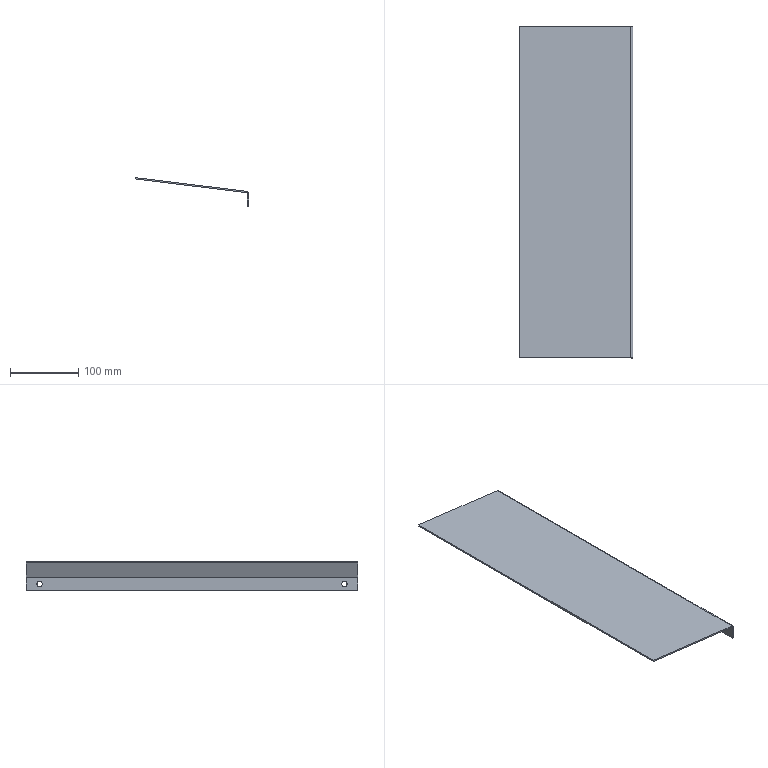Part | STEP file | JBJ-P-1006-09 | 1 solid | 16 faces | box 167 x 488 x 42.231 mm | volume 182511 mm3 | plane 12 | cylinder 4 | commonest cylinder face diameters 8 x2 3 x1 7 x1
STEP:
#1=CARTESIAN_POINT('',(163.,488.,-1.327));
#2=VERTEX_POINT('',#1);
#3=CARTESIAN_POINT('',(165.,488.,-1.327));
#4=VERTEX_POINT('',#3);
#5=CARTESIAN_POINT('',(163.,488.,-1.327));
#6=DIRECTION('',(1.,0.,0.));
#7=VECTOR('',#6,1000.);
#8=LINE('',#5,#7);
#9=EDGE_CURVE('',#2,#4,#8,.T.);
#10=ORIENTED_EDGE('',*,*,#9,.F.);
#11=CARTESIAN_POINT('',(161.683,488.,0.1616));
#12=VERTEX_POINT('',#11);
#13=CARTESIAN_POINT('',(161.5,488.,-1.327));
#14=DIRECTION('',(0.,1.,0.));
#15=DIRECTION('',(0.,0.,-1.));
#16=AXIS2_PLACEMENT_3D('',#13,#14,#15);
#17=CIRCLE('',#16,1.5);
#18=EDGE_CURVE('',#12,#2,#17,.T.);
#19=ORIENTED_EDGE('',*,*,#18,.F.);
#20=CARTESIAN_POINT('',(161.926,488.,2.147));
#21=VERTEX_POINT('',#20);
#22=CARTESIAN_POINT('',(161.926,488.,2.147));
#23=DIRECTION('',(-0.1218,0.,-0.9926));
#24=VECTOR('',#23,1000.);
#25=LINE('',#22,#24);
#26=EDGE_CURVE('',#21,#12,#25,.T.);
#27=ORIENTED_EDGE('',*,*,#26,.F.);
#28=CARTESIAN_POINT('',(161.5,488.,-1.327));
#29=DIRECTION('',(0.,1.,0.));
#30=DIRECTION('',(1.,0.,0.));
#31=AXIS2_PLACEMENT_3D('',#28,#29,#30);
#32=CIRCLE('',#31,3.5);
#33=EDGE_CURVE('',#21,#4,#32,.T.);
#34=ORIENTED_EDGE('',*,*,#33,.T.);
#35=EDGE_LOOP('',(#10,#19,#27,#34));
#36=FACE_OUTER_BOUND('',#35,.T.);
#37=CARTESIAN_POINT('',(163.,488.,-1.327));
#38=DIRECTION('',(0.,1.,0.));
#39=DIRECTION('',(0.,0.,1.));
#40=AXIS2_PLACEMENT_3D('',#37,#38,#39);
#41=PLANE('',#40);
#42=ADVANCED_FACE('',(#36),#41,.T.);
#43=CARTESIAN_POINT('',(163.,488.,-20.));
#44=VERTEX_POINT('',#43);
#45=CARTESIAN_POINT('',(163.,488.,0.));
#46=DIRECTION('',(0.,0.,-1.));
#47=VECTOR('',#46,1000.);
#48=LINE('',#45,#47);
#49=EDGE_CURVE('',#2,#44,#48,.T.);
#50=ORIENTED_EDGE('',*,*,#49,.F.);
#51=ORIENTED_EDGE('',*,*,#9,.T.);
#52=CARTESIAN_POINT('',(165.,488.,-20.));
#53=VERTEX_POINT('',#52);
#54=CARTESIAN_POINT('',(165.,488.,0.));
#55=DIRECTION('',(0.,0.,-1.));
#56=VECTOR('',#55,1000.);
#57=LINE('',#54,#56);
#58=EDGE_CURVE('',#4,#53,#57,.T.);
#59=ORIENTED_EDGE('',*,*,#58,.T.);
#60=CARTESIAN_POINT('',(163.,488.,-20.));
#61=DIRECTION('',(1.,0.,0.));
#62=VECTOR('',#61,1000.);
#63=LINE('',#60,#62);
#64=EDGE_CURVE('',#44,#53,#63,.T.);
#65=ORIENTED_EDGE('',*,*,#64,.F.);
#66=EDGE_LOOP('',(#50,#51,#59,#65));
#67=FACE_OUTER_BOUND('',#66,.T.);
#68=CARTESIAN_POINT('',(161.926,488.,2.147));
#69=DIRECTION('',(0.,1.,0.));
#70=DIRECTION('',(0.,0.,1.));
#71=AXIS2_PLACEMENT_3D('',#68,#69,#70);
#72=PLANE('',#71);
#73=ADVANCED_FACE('',(#67),#72,.T.);
#74=CARTESIAN_POINT('',(161.683,0.,0.1616));
#75=VERTEX_POINT('',#74);
#76=CARTESIAN_POINT('',(161.926,0.,2.147));
#77=VERTEX_POINT('',#76);
#78=CARTESIAN_POINT('',(161.683,0.,0.1616));
#79=DIRECTION('',(0.1218,0.,0.9926));
#80=VECTOR('',#79,1000.);
#81=LINE('',#78,#80);
#82=EDGE_CURVE('',#75,#77,#81,.T.);
#83=ORIENTED_EDGE('',*,*,#82,.F.);
#84=CARTESIAN_POINT('',(163.,0.,-1.327));
#85=VERTEX_POINT('',#84);
#86=CARTESIAN_POINT('',(161.5,0.,-1.327));
#87=DIRECTION('',(0.,1.,0.));
#88=DIRECTION('',(0.,0.,-1.));
#89=AXIS2_PLACEMENT_3D('',#86,#87,#88);
#90=CIRCLE('',#89,1.5);
#91=EDGE_CURVE('',#75,#85,#90,.T.);
#92=ORIENTED_EDGE('',*,*,#91,.T.);
#93=CARTESIAN_POINT('',(165.,0.,-1.327));
#94=VERTEX_POINT('',#93);
#95=CARTESIAN_POINT('',(165.,0.,-1.327));
#96=DIRECTION('',(-1.,0.,0.));
#97=VECTOR('',#96,1000.);
#98=LINE('',#95,#97);
#99=EDGE_CURVE('',#94,#85,#98,.T.);
#100=ORIENTED_EDGE('',*,*,#99,.F.);
#101=CARTESIAN_POINT('',(161.5,0.,-1.327));
#102=DIRECTION('',(0.,1.,0.));
#103=DIRECTION('',(1.,0.,0.));
#104=AXIS2_PLACEMENT_3D('',#101,#102,#103);
#105=CIRCLE('',#104,3.5);
#106=EDGE_CURVE('',#77,#94,#105,.T.);
#107=ORIENTED_EDGE('',*,*,#106,.F.);
#108=EDGE_LOOP('',(#83,#92,#100,#107));
#109=FACE_OUTER_BOUND('',#108,.T.);
#110=CARTESIAN_POINT('',(161.683,0.,0.1616));
#111=DIRECTION('',(0.,-1.,0.));
#112=DIRECTION('',(0.,0.,-1.));
#113=AXIS2_PLACEMENT_3D('',#110,#111,#112);
#114=PLANE('',#113);
#115=ADVANCED_FACE('',(#109),#114,.T.);
#116=CARTESIAN_POINT('',(-2.,0.,20.245));
#117=VERTEX_POINT('',#116);
#118=CARTESIAN_POINT('',(-2.,0.,20.245));
#119=DIRECTION('',(0.9926,0.,-0.1218));
#120=VECTOR('',#119,1000.);
#121=LINE('',#118,#120);
#122=EDGE_CURVE('',#117,#75,#121,.T.);
#123=ORIENTED_EDGE('',*,*,#122,.T.);
#124=ORIENTED_EDGE('',*,*,#82,.T.);
#125=CARTESIAN_POINT('',(-1.756,0.,22.231));
#126=VERTEX_POINT('',#125);
#127=CARTESIAN_POINT('',(-1.756,0.,22.231));
#128=DIRECTION('',(0.9926,0.,-0.1218));
#129=VECTOR('',#128,1000.);
#130=LINE('',#127,#129);
#131=EDGE_CURVE('',#126,#77,#130,.T.);
#132=ORIENTED_EDGE('',*,*,#131,.F.);
#133=CARTESIAN_POINT('',(-1.756,0.,22.231));
#134=DIRECTION('',(-0.1218,0.,-0.9926));
#135=VECTOR('',#134,1000.);
#136=LINE('',#133,#135);
#137=EDGE_CURVE('',#126,#117,#136,.T.);
#138=ORIENTED_EDGE('',*,*,#137,.T.);
#139=EDGE_LOOP('',(#123,#124,#132,#138));
#140=FACE_OUTER_BOUND('',#139,.T.);
#141=CARTESIAN_POINT('',(165.,0.,-1.327));
#142=DIRECTION('',(0.,-1.,0.));
#143=DIRECTION('',(0.,0.,-1.));
#144=AXIS2_PLACEMENT_3D('',#141,#142,#143);
#145=PLANE('',#144);
#146=ADVANCED_FACE('',(#140),#145,.T.);
#147=CARTESIAN_POINT('',(165.,468.,-6.664));
#148=VERTEX_POINT('',#147);
#149=CARTESIAN_POINT('',(165.,468.,-10.664));
#150=DIRECTION('',(-1.,0.,0.));
#151=DIRECTION('',(0.,0.,1.));
#152=AXIS2_PLACEMENT_3D('',#149,#150,#151);
#153=CIRCLE('',#152,4.);
#154=EDGE_CURVE('',#148,#148,#153,.T.);
#155=ORIENTED_EDGE('',*,*,#154,.T.);
#156=EDGE_LOOP('',(#155));
#157=FACE_BOUND('',#156,.T.);
#158=CARTESIAN_POINT('',(165.,20.,-6.664));
#159=VERTEX_POINT('',#158);
#160=CARTESIAN_POINT('',(165.,20.,-10.664));
#161=DIRECTION('',(-1.,0.,0.));
#162=DIRECTION('',(0.,0.,1.));
#163=AXIS2_PLACEMENT_3D('',#160,#161,#162);
#164=CIRCLE('',#163,4.);
#165=EDGE_CURVE('',#159,#159,#164,.T.);
#166=ORIENTED_EDGE('',*,*,#165,.T.);
#167=EDGE_LOOP('',(#166));
#168=FACE_BOUND('',#167,.T.);
#169=CARTESIAN_POINT('',(165.,0.,-20.));
#170=VERTEX_POINT('',#169);
#171=CARTESIAN_POINT('',(165.,0.,0.));
#172=DIRECTION('',(0.,0.,-1.));
#173=VECTOR('',#172,1000.);
#174=LINE('',#171,#173);
#175=EDGE_CURVE('',#94,#170,#174,.T.);
#176=ORIENTED_EDGE('',*,*,#175,.T.);
#177=CARTESIAN_POINT('',(165.,488.,-20.));
#178=DIRECTION('',(0.,-1.,0.));
#179=VECTOR('',#178,1000.);
#180=LINE('',#177,#179);
#181=EDGE_CURVE('',#53,#170,#180,.T.);
#182=ORIENTED_EDGE('',*,*,#181,.F.);
#183=ORIENTED_EDGE('',*,*,#58,.F.);
#184=CARTESIAN_POINT('',(165.,488.,-1.327));
#185=DIRECTION('',(0.,-1.,0.));
#186=VECTOR('',#185,1000.);
#187=LINE('',#184,#186);
#188=EDGE_CURVE('',#4,#94,#187,.T.);
#189=ORIENTED_EDGE('',*,*,#188,.T.);
#190=EDGE_LOOP('',(#176,#182,#183,#189));
#191=FACE_OUTER_BOUND('',#190,.T.);
#192=CARTESIAN_POINT('',(165.,488.,0.));
#193=DIRECTION('',(-1.,0.,0.));
#194=DIRECTION('',(0.,0.,1.));
#195=AXIS2_PLACEMENT_3D('',#192,#193,#194);
#196=PLANE('',#195);
#197=ADVANCED_FACE('',(#157,#168,#191),#196,.F.);
#198=CARTESIAN_POINT('',(163.,0.,-20.));
#199=VERTEX_POINT('',#198);
#200=CARTESIAN_POINT('',(163.,0.,-20.));
#201=DIRECTION('',(1.,0.,0.));
#202=VECTOR('',#201,1000.);
#203=LINE('',#200,#202);
#204=EDGE_CURVE('',#199,#170,#203,.T.);
#205=ORIENTED_EDGE('',*,*,#204,.F.);
#206=CARTESIAN_POINT('',(163.,488.,-20.));
#207=DIRECTION('',(0.,-1.,0.));
#208=VECTOR('',#207,1000.);
#209=LINE('',#206,#208);
#210=EDGE_CURVE('',#44,#199,#209,.T.);
#211=ORIENTED_EDGE('',*,*,#210,.F.);
#212=ORIENTED_EDGE('',*,*,#64,.T.);
#213=ORIENTED_EDGE('',*,*,#181,.T.);
#214=EDGE_LOOP('',(#205,#211,#212,#213));
#215=FACE_OUTER_BOUND('',#214,.T.);
#216=CARTESIAN_POINT('',(163.,488.,-20.));
#217=DIRECTION('',(0.,0.,-1.));
#218=DIRECTION('',(-1.,0.,0.));
#219=AXIS2_PLACEMENT_3D('',#216,#217,#218);
#220=PLANE('',#219);
#221=ADVANCED_FACE('',(#215),#220,.T.);
#222=CARTESIAN_POINT('',(163.,468.,-6.664));
#223=VERTEX_POINT('',#222);
#224=CARTESIAN_POINT('',(163.,468.,-10.664));
#225=DIRECTION('',(-1.,0.,0.));
#226=DIRECTION('',(0.,0.,1.));
#227=AXIS2_PLACEMENT_3D('',#224,#225,#226);
#228=CIRCLE('',#227,4.);
#229=EDGE_CURVE('',#223,#223,#228,.T.);
#230=ORIENTED_EDGE('',*,*,#229,.F.);
#231=EDGE_LOOP('',(#230));
#232=FACE_BOUND('',#231,.T.);
#233=CARTESIAN_POINT('',(163.,20.,-6.664));
#234=VERTEX_POINT('',#233);
#235=CARTESIAN_POINT('',(163.,20.,-10.664));
#236=DIRECTION('',(-1.,0.,0.));
#237=DIRECTION('',(0.,0.,1.));
#238=AXIS2_PLACEMENT_3D('',#235,#236,#237);
#239=CIRCLE('',#238,4.);
#240=EDGE_CURVE('',#234,#234,#239,.T.);
#241=ORIENTED_EDGE('',*,*,#240,.F.);
#242=EDGE_LOOP('',(#241));
#243=FACE_BOUND('',#242,.T.);
#244=CARTESIAN_POINT('',(163.,0.,0.));
#245=DIRECTION('',(0.,0.,-1.));
#246=VECTOR('',#245,1000.);
#247=LINE('',#244,#246);
#248=EDGE_CURVE('',#85,#199,#247,.T.);
#249=ORIENTED_EDGE('',*,*,#248,.F.);
#250=CARTESIAN_POINT('',(163.,488.,-1.327));
#251=DIRECTION('',(0.,-1.,0.));
#252=VECTOR('',#251,1000.);
#253=LINE('',#250,#252);
#254=EDGE_CURVE('',#2,#85,#253,.T.);
#255=ORIENTED_EDGE('',*,*,#254,.F.);
#256=ORIENTED_EDGE('',*,*,#49,.T.);
#257=ORIENTED_EDGE('',*,*,#210,.T.);
#258=EDGE_LOOP('',(#249,#255,#256,#257));
#259=FACE_OUTER_BOUND('',#258,.T.);
#260=CARTESIAN_POINT('',(163.,488.,0.));
#261=DIRECTION('',(-1.,0.,0.));
#262=DIRECTION('',(0.,0.,1.));
#263=AXIS2_PLACEMENT_3D('',#260,#261,#262);
#264=PLANE('',#263);
#265=ADVANCED_FACE('',(#232,#243,#259),#264,.T.);
#266=ORIENTED_EDGE('',*,*,#91,.F.);
#267=CARTESIAN_POINT('',(161.683,488.,0.1616));
#268=DIRECTION('',(0.,-1.,0.));
#269=VECTOR('',#268,1000.);
#270=LINE('',#267,#269);
#271=EDGE_CURVE('',#12,#75,#270,.T.);
#272=ORIENTED_EDGE('',*,*,#271,.F.);
#273=ORIENTED_EDGE('',*,*,#18,.T.);
#274=ORIENTED_EDGE('',*,*,#254,.T.);
#275=EDGE_LOOP('',(#266,#272,#273,#274));
#276=FACE_OUTER_BOUND('',#275,.T.);
#277=CARTESIAN_POINT('',(161.5,488.,-1.327));
#278=DIRECTION('',(0.,-1.,0.));
#279=DIRECTION('',(0.,0.,-1.));
#280=AXIS2_PLACEMENT_3D('',#277,#278,#279);
#281=CYLINDRICAL_SURFACE('',#280,1.5);
#282=ADVANCED_FACE('',(#276),#281,.F.);
#283=ORIENTED_EDGE('',*,*,#122,.F.);
#284=CARTESIAN_POINT('',(-2.,488.,20.245));
#285=VERTEX_POINT('',#284);
#286=CARTESIAN_POINT('',(-2.,488.,20.245));
#287=DIRECTION('',(0.,-1.,0.));
#288=VECTOR('',#287,1000.);
#289=LINE('',#286,#288);
#290=EDGE_CURVE('',#285,#117,#289,.T.);
#291=ORIENTED_EDGE('',*,*,#290,.F.);
#292=CARTESIAN_POINT('',(-2.,488.,20.245));
#293=DIRECTION('',(0.9926,0.,-0.1218));
#294=VECTOR('',#293,1000.);
#295=LINE('',#292,#294);
#296=EDGE_CURVE('',#285,#12,#295,.T.);
#297=ORIENTED_EDGE('',*,*,#296,.T.);
#298=ORIENTED_EDGE('',*,*,#271,.T.);
#299=EDGE_LOOP('',(#283,#291,#297,#298));
#300=FACE_OUTER_BOUND('',#299,.T.);
#301=CARTESIAN_POINT('',(-2.,488.,20.245));
#302=DIRECTION('',(-0.1218,0.,-0.9926));
#303=DIRECTION('',(-0.9926,0.,0.1218));
#304=AXIS2_PLACEMENT_3D('',#301,#302,#303);
#305=PLANE('',#304);
#306=ADVANCED_FACE('',(#300),#305,.T.);
#307=ORIENTED_EDGE('',*,*,#137,.F.);
#308=CARTESIAN_POINT('',(-1.756,488.,22.231));
#309=VERTEX_POINT('',#308);
#310=CARTESIAN_POINT('',(-1.756,488.,22.231));
#311=DIRECTION('',(0.,-1.,0.));
#312=VECTOR('',#311,1000.);
#313=LINE('',#310,#312);
#314=EDGE_CURVE('',#309,#126,#313,.T.);
#315=ORIENTED_EDGE('',*,*,#314,.F.);
#316=CARTESIAN_POINT('',(-1.756,488.,22.231));
#317=DIRECTION('',(-0.1218,0.,-0.9926));
#318=VECTOR('',#317,1000.);
#319=LINE('',#316,#318);
#320=EDGE_CURVE('',#309,#285,#319,.T.);
#321=ORIENTED_EDGE('',*,*,#320,.T.);
#322=ORIENTED_EDGE('',*,*,#290,.T.);
#323=EDGE_LOOP('',(#307,#315,#321,#322));
#324=FACE_OUTER_BOUND('',#323,.T.);
#325=CARTESIAN_POINT('',(-1.756,488.,22.231));
#326=DIRECTION('',(-0.9926,0.,0.1218));
#327=DIRECTION('',(0.1218,0.,0.9926));
#328=AXIS2_PLACEMENT_3D('',#325,#326,#327);
#329=PLANE('',#328);
#330=ADVANCED_FACE('',(#324),#329,.T.);
#331=ORIENTED_EDGE('',*,*,#131,.T.);
#332=CARTESIAN_POINT('',(161.926,488.,2.147));
#333=DIRECTION('',(0.,-1.,0.));
#334=VECTOR('',#333,1000.);
#335=LINE('',#332,#334);
#336=EDGE_CURVE('',#21,#77,#335,.T.);
#337=ORIENTED_EDGE('',*,*,#336,.F.);
#338=CARTESIAN_POINT('',(-1.756,488.,22.231));
#339=DIRECTION('',(0.9926,0.,-0.1218));
#340=VECTOR('',#339,1000.);
#341=LINE('',#338,#340);
#342=EDGE_CURVE('',#309,#21,#341,.T.);
#343=ORIENTED_EDGE('',*,*,#342,.F.);
#344=ORIENTED_EDGE('',*,*,#314,.T.);
#345=EDGE_LOOP('',(#331,#337,#343,#344));
#346=FACE_OUTER_BOUND('',#345,.T.);
#347=CARTESIAN_POINT('',(-1.756,488.,22.231));
#348=DIRECTION('',(-0.1218,0.,-0.9926));
#349=DIRECTION('',(-0.9926,0.,0.1218));
#350=AXIS2_PLACEMENT_3D('',#347,#348,#349);
#351=PLANE('',#350);
#352=ADVANCED_FACE('',(#346),#351,.F.);
#353=ORIENTED_EDGE('',*,*,#106,.T.);
#354=ORIENTED_EDGE('',*,*,#188,.F.);
#355=ORIENTED_EDGE('',*,*,#33,.F.);
#356=ORIENTED_EDGE('',*,*,#336,.T.);
#357=EDGE_LOOP('',(#353,#354,#355,#356));
#358=FACE_OUTER_BOUND('',#357,.T.);
#359=CARTESIAN_POINT('',(161.5,488.,-1.327));
#360=DIRECTION('',(0.,-1.,0.));
#361=DIRECTION('',(0.,0.,-1.));
#362=AXIS2_PLACEMENT_3D('',#359,#360,#361);
#363=CYLINDRICAL_SURFACE('',#362,3.5);
#364=ADVANCED_FACE('',(#358),#363,.T.);
#365=ORIENTED_EDGE('',*,*,#342,.T.);
#366=ORIENTED_EDGE('',*,*,#26,.T.);
#367=ORIENTED_EDGE('',*,*,#296,.F.);
#368=ORIENTED_EDGE('',*,*,#320,.F.);
#369=EDGE_LOOP('',(#365,#366,#367,#368));
#370=FACE_OUTER_BOUND('',#369,.T.);
#371=CARTESIAN_POINT('',(161.5,488.,-1.327));
#372=DIRECTION('',(0.,-1.,0.));
#373=DIRECTION('',(-1.,0.,0.));
#374=AXIS2_PLACEMENT_3D('',#371,#372,#373);
#375=PLANE('',#374);
#376=ADVANCED_FACE('',(#370),#375,.F.);
#377=ORIENTED_EDGE('',*,*,#175,.F.);
#378=ORIENTED_EDGE('',*,*,#99,.T.);
#379=ORIENTED_EDGE('',*,*,#248,.T.);
#380=ORIENTED_EDGE('',*,*,#204,.T.);
#381=EDGE_LOOP('',(#377,#378,#379,#380));
#382=FACE_OUTER_BOUND('',#381,.T.);
#383=CARTESIAN_POINT('',(161.5,0.,-1.327));
#384=DIRECTION('',(0.,-1.,0.));
#385=DIRECTION('',(-1.,0.,0.));
#386=AXIS2_PLACEMENT_3D('',#383,#384,#385);
#387=PLANE('',#386);
#388=ADVANCED_FACE('',(#382),#387,.T.);
#389=ORIENTED_EDGE('',*,*,#240,.T.);
#390=EDGE_LOOP('',(#389));
#391=FACE_OUTER_BOUND('',#390,.T.);
#392=ORIENTED_EDGE('',*,*,#165,.F.);
#393=EDGE_LOOP('',(#392));
#394=FACE_OUTER_BOUND('',#393,.T.);
#395=CARTESIAN_POINT('',(173.,20.,-10.664));
#396=DIRECTION('',(-1.,0.,0.));
#397=DIRECTION('',(0.,0.,1.));
#398=AXIS2_PLACEMENT_3D('',#395,#396,#397);
#399=CYLINDRICAL_SURFACE('',#398,4.);
#400=ADVANCED_FACE('',(#391,#394),#399,.F.);
#401=ORIENTED_EDGE('',*,*,#229,.T.);
#402=EDGE_LOOP('',(#401));
#403=FACE_OUTER_BOUND('',#402,.T.);
#404=ORIENTED_EDGE('',*,*,#154,.F.);
#405=EDGE_LOOP('',(#404));
#406=FACE_OUTER_BOUND('',#405,.T.);
#407=CARTESIAN_POINT('',(173.,468.,-10.664));
#408=DIRECTION('',(-1.,0.,0.));
#409=DIRECTION('',(0.,0.,1.));
#410=AXIS2_PLACEMENT_3D('',#407,#408,#409);
#411=CYLINDRICAL_SURFACE('',#410,4.);
#412=ADVANCED_FACE('',(#403,#406),#411,.F.);
#413=CLOSED_SHELL('',(#42,#73,#115,#146,#197,#221,#265,#282,#306,#330,#352,#364,#376,#388,#400,#412));
#414=MANIFOLD_SOLID_BREP('',#413);
#415=CARTESIAN_POINT('',(0.,0.,0.));
#416=DIRECTION('',(0.,0.,1.));
#417=DIRECTION('',(1.,0.,0.));
#418=AXIS2_PLACEMENT_3D('',#415,#416,#417);
#419=(LENGTH_UNIT()NAMED_UNIT(*)SI_UNIT(.MILLI.,.METRE.));
#420=UNCERTAINTY_MEASURE_WITH_UNIT(LENGTH_MEASURE(0.00001),#419,'','');
#421=(NAMED_UNIT(*)PLANE_ANGLE_UNIT()SI_UNIT($,.RADIAN.));
#422=(NAMED_UNIT(*)SI_UNIT($,.STERADIAN.)SOLID_ANGLE_UNIT());
#423=(GEOMETRIC_REPRESENTATION_CONTEXT(3)GLOBAL_UNCERTAINTY_ASSIGNED_CONTEXT((#420))GLOBAL_UNIT_ASSIGNED_CONTEXT((#419,#421,#422))REPRESENTATION_CONTEXT('',''));
#424=ADVANCED_BREP_SHAPE_REPRESENTATION('',(#414,#418),#423);